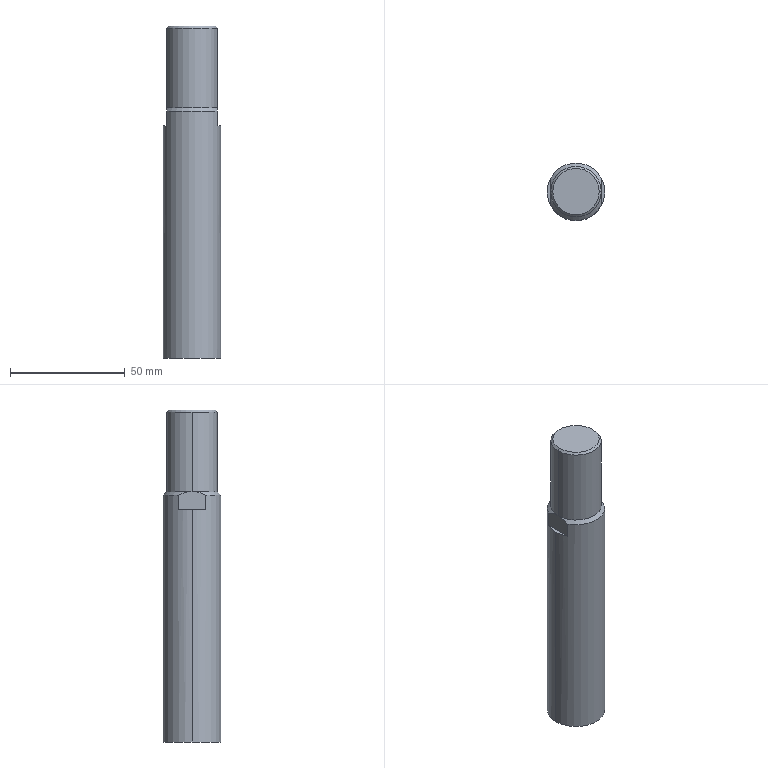Part | STEP file | A_CDQ2A80-100DM-F9NV (Rod) | 1 solid | 14 faces | box 25 x 25 x 144.5 mm | volume 66720 mm3 | cone 4 | cylinder 4 | plane 4 | spline 2 | commonest cylinder face diameters 22 x2 25 x2
STEP:
#1=CARTESIAN_POINT('',(0.,0.,0.));
#2=DIRECTION('',(0.,0.,1.));
#3=DIRECTION('',(1.,0.,0.));
#4=AXIS2_PLACEMENT_3D('',#1,#2,#3);
#5=CARTESIAN_POINT('',(-10.105,0.,43.5));
#6=VERTEX_POINT('',#5);
#7=CARTESIAN_POINT('',(10.105,0.,43.5));
#8=VERTEX_POINT('',#7);
#9=CARTESIAN_POINT('',(0.,0.,43.5));
#10=DIRECTION('',(0.,0.,-1.));
#11=DIRECTION('',(-1.,0.,0.));
#12=AXIS2_PLACEMENT_3D('',#9,#10,#11);
#13=CIRCLE('',#12,10.105);
#14=CARTESIAN_POINT('',(0.,0.,43.5));
#15=DIRECTION('',(0.,0.,-1.));
#16=DIRECTION('',(-1.,0.,0.));
#17=AXIS2_PLACEMENT_3D('',#14,#15,#16);
#18=CONICAL_SURFACE('',#17,10.105,0.7854);
#19=CARTESIAN_POINT('',(0.,0.));
#20=DIRECTION('',(1.,0.));
#21=VECTOR('',#20,1.);
#22=LINE('',#19,#21);
#23=(GEOMETRIC_REPRESENTATION_CONTEXT(2)PARAMETRIC_REPRESENTATION_CONTEXT()REPRESENTATION_CONTEXT('',''));
#24=DEFINITIONAL_REPRESENTATION('',(#22),#23);
#25=PCURVE('',#18,#24);
#26=CARTESIAN_POINT('',(10.226,-10.105,43.5));
#27=DIRECTION('',(0.,0.,1.));
#28=DIRECTION('',(0.,1.,0.));
#29=AXIS2_PLACEMENT_3D('',#26,#27,#28);
#30=PLANE('',#29);
#31=CARTESIAN_POINT('',(10.105,20.331));
#32=CARTESIAN_POINT('',(27.607,20.331));
#33=CARTESIAN_POINT('',(18.856,5.174));
#34=CARTESIAN_POINT('',(10.105,-9.984));
#35=CARTESIAN_POINT('',(1.354,5.174));
#36=CARTESIAN_POINT('',(-7.397,20.331));
#37=CARTESIAN_POINT('',(10.105,20.331));
#38=(BOUNDED_CURVE()B_SPLINE_CURVE(2,(#31,#32,#33,#34,#35,#36,#37),.UNSPECIFIED.,.T.,.F.)B_SPLINE_CURVE_WITH_KNOTS((1,2,2,2,2,1),(-2.094,0.,2.094,4.189,6.283,8.378),.UNSPECIFIED.)CURVE()GEOMETRIC_REPRESENTATION_ITEM()RATIONAL_B_SPLINE_CURVE((1.,0.5,1.,0.5,1.,0.5,1.))REPRESENTATION_ITEM(''));
#39=(GEOMETRIC_REPRESENTATION_CONTEXT(2)PARAMETRIC_REPRESENTATION_CONTEXT()REPRESENTATION_CONTEXT('',''));
#40=DEFINITIONAL_REPRESENTATION('',(#38),#39);
#41=PCURVE('',#30,#40);
#42=SURFACE_CURVE('',#13,(#25,#41),.PCURVE_S1.);
#43=EDGE_CURVE('',#6,#8,#42,.T.);
#44=ORIENTED_EDGE('',*,*,#43,.T.);
#45=CARTESIAN_POINT('',(11.,0.,42.605));
#46=VERTEX_POINT('',#45);
#47=CARTESIAN_POINT('',(10.105,0.,43.5));
#48=DIRECTION('',(0.7071,0.,-0.7071));
#49=VECTOR('',#48,1.);
#50=LINE('',#47,#49);
#51=CARTESIAN_POINT('',(3.142,0.));
#52=DIRECTION('',(0.,1.));
#53=VECTOR('',#52,1.);
#54=LINE('',#51,#53);
#55=(GEOMETRIC_REPRESENTATION_CONTEXT(2)PARAMETRIC_REPRESENTATION_CONTEXT()REPRESENTATION_CONTEXT('',''));
#56=DEFINITIONAL_REPRESENTATION('',(#54),#55);
#57=PCURVE('',#18,#56);
#58=CARTESIAN_POINT('',(0.,0.,43.5));
#59=DIRECTION('',(0.,0.,-1.));
#60=DIRECTION('',(-1.,0.,0.));
#61=AXIS2_PLACEMENT_3D('',#58,#59,#60);
#62=CONICAL_SURFACE('',#61,10.105,0.7854);
#63=CARTESIAN_POINT('',(3.142,0.));
#64=DIRECTION('',(0.,1.));
#65=VECTOR('',#64,1.);
#66=LINE('',#63,#65);
#67=(GEOMETRIC_REPRESENTATION_CONTEXT(2)PARAMETRIC_REPRESENTATION_CONTEXT()REPRESENTATION_CONTEXT('',''));
#68=DEFINITIONAL_REPRESENTATION('',(#66),#67);
#69=PCURVE('',#62,#68);
#70=SURFACE_CURVE('',#50,(#57,#69),.PCURVE_S1.);
#71=EDGE_CURVE('',#8,#46,#70,.T.);
#72=ORIENTED_EDGE('',*,*,#71,.T.);
#73=CARTESIAN_POINT('',(-11.,0.,42.605));
#74=VERTEX_POINT('',#73);
#75=CARTESIAN_POINT('',(0.,0.,42.605));
#76=DIRECTION('',(0.,0.,1.));
#77=DIRECTION('',(0.,1.,0.));
#78=AXIS2_PLACEMENT_3D('',#75,#76,#77);
#79=CIRCLE('',#78,11.);
#80=CARTESIAN_POINT('',(7.854,0.895));
#81=DIRECTION('',(-1.,0.));
#82=VECTOR('',#81,1.);
#83=LINE('',#80,#82);
#84=(GEOMETRIC_REPRESENTATION_CONTEXT(2)PARAMETRIC_REPRESENTATION_CONTEXT()REPRESENTATION_CONTEXT('',''));
#85=DEFINITIONAL_REPRESENTATION('',(#83),#84);
#86=PCURVE('',#18,#85);
#87=CARTESIAN_POINT('',(0.,0.,42.605));
#88=DIRECTION('',(0.,0.,1.));
#89=DIRECTION('',(1.,0.,0.));
#90=AXIS2_PLACEMENT_3D('',#87,#88,#89);
#91=CYLINDRICAL_SURFACE('',#90,11.);
#92=CARTESIAN_POINT('',(-4.712,0.));
#93=DIRECTION('',(1.,0.));
#94=VECTOR('',#93,1.);
#95=LINE('',#92,#94);
#96=(GEOMETRIC_REPRESENTATION_CONTEXT(2)PARAMETRIC_REPRESENTATION_CONTEXT()REPRESENTATION_CONTEXT('',''));
#97=DEFINITIONAL_REPRESENTATION('',(#95),#96);
#98=PCURVE('',#91,#97);
#99=SURFACE_CURVE('',#79,(#86,#98),.PCURVE_S1.);
#100=EDGE_CURVE('',#46,#74,#99,.T.);
#101=ORIENTED_EDGE('',*,*,#100,.T.);
#102=CARTESIAN_POINT('',(-10.105,0.,43.5));
#103=DIRECTION('',(-0.7071,0.,-0.7071));
#104=VECTOR('',#103,1.);
#105=LINE('',#102,#104);
#106=CARTESIAN_POINT('',(0.,0.));
#107=DIRECTION('',(0.,1.));
#108=VECTOR('',#107,1.);
#109=LINE('',#106,#108);
#110=(GEOMETRIC_REPRESENTATION_CONTEXT(2)PARAMETRIC_REPRESENTATION_CONTEXT()REPRESENTATION_CONTEXT('',''));
#111=DEFINITIONAL_REPRESENTATION('',(#109),#110);
#112=PCURVE('',#18,#111);
#113=CARTESIAN_POINT('',(6.283,0.));
#114=DIRECTION('',(0.,1.));
#115=VECTOR('',#114,1.);
#116=LINE('',#113,#115);
#117=(GEOMETRIC_REPRESENTATION_CONTEXT(2)PARAMETRIC_REPRESENTATION_CONTEXT()REPRESENTATION_CONTEXT('',''));
#118=DEFINITIONAL_REPRESENTATION('',(#116),#117);
#119=PCURVE('',#62,#118);
#120=SURFACE_CURVE('',#105,(#112,#119),.PCURVE_S1.);
#121=EDGE_CURVE('',#6,#74,#120,.T.);
#122=ORIENTED_EDGE('',*,*,#121,.F.);
#123=EDGE_LOOP('',(#44,#72,#101,#122));
#124=FACE_BOUND('',#123,.T.);
#125=ADVANCED_FACE('',(#124),#18,.T.);
#126=CARTESIAN_POINT('',(11.,0.,8.));
#127=VERTEX_POINT('',#126);
#128=CARTESIAN_POINT('',(-11.,0.,8.));
#129=VERTEX_POINT('',#128);
#130=CARTESIAN_POINT('',(0.,0.,8.));
#131=DIRECTION('',(0.,0.,1.));
#132=DIRECTION('',(0.,1.,0.));
#133=AXIS2_PLACEMENT_3D('',#130,#131,#132);
#134=CIRCLE('',#133,11.);
#135=CARTESIAN_POINT('',(-4.712,-34.605));
#136=DIRECTION('',(1.,0.));
#137=VECTOR('',#136,1.);
#138=LINE('',#135,#137);
#139=(GEOMETRIC_REPRESENTATION_CONTEXT(2)PARAMETRIC_REPRESENTATION_CONTEXT()REPRESENTATION_CONTEXT('',''));
#140=DEFINITIONAL_REPRESENTATION('',(#138),#139);
#141=PCURVE('',#91,#140);
#142=CARTESIAN_POINT('',(0.,0.,8.));
#143=DIRECTION('',(0.,0.,-1.));
#144=DIRECTION('',(-1.,0.,0.));
#145=AXIS2_PLACEMENT_3D('',#142,#143,#144);
#146=CONICAL_SURFACE('',#145,11.,0.7854);
#147=CARTESIAN_POINT('',(7.854,0.));
#148=DIRECTION('',(-1.,0.));
#149=VECTOR('',#148,1.);
#150=LINE('',#147,#149);
#151=(GEOMETRIC_REPRESENTATION_CONTEXT(2)PARAMETRIC_REPRESENTATION_CONTEXT()REPRESENTATION_CONTEXT('',''));
#152=DEFINITIONAL_REPRESENTATION('',(#150),#151);
#153=PCURVE('',#146,#152);
#154=SURFACE_CURVE('',#134,(#141,#153),.PCURVE_S1.);
#155=EDGE_CURVE('',#127,#129,#154,.T.);
#156=ORIENTED_EDGE('',*,*,#155,.T.);
#157=CARTESIAN_POINT('',(-11.,0.,42.605));
#158=DIRECTION('',(0.,0.,1.));
#159=VECTOR('',#158,1.);
#160=LINE('',#157,#159);
#161=CARTESIAN_POINT('',(3.142,0.));
#162=DIRECTION('',(0.,1.));
#163=VECTOR('',#162,1.);
#164=LINE('',#161,#163);
#165=(GEOMETRIC_REPRESENTATION_CONTEXT(2)PARAMETRIC_REPRESENTATION_CONTEXT()REPRESENTATION_CONTEXT('',''));
#166=DEFINITIONAL_REPRESENTATION('',(#164),#165);
#167=PCURVE('',#91,#166);
#168=CARTESIAN_POINT('',(0.,0.,42.605));
#169=DIRECTION('',(0.,0.,1.));
#170=DIRECTION('',(1.,0.,0.));
#171=AXIS2_PLACEMENT_3D('',#168,#169,#170);
#172=CYLINDRICAL_SURFACE('',#171,11.);
#173=CARTESIAN_POINT('',(3.142,0.));
#174=DIRECTION('',(0.,1.));
#175=VECTOR('',#174,1.);
#176=LINE('',#173,#175);
#177=(GEOMETRIC_REPRESENTATION_CONTEXT(2)PARAMETRIC_REPRESENTATION_CONTEXT()REPRESENTATION_CONTEXT('',''));
#178=DEFINITIONAL_REPRESENTATION('',(#176),#177);
#179=PCURVE('',#172,#178);
#180=SURFACE_CURVE('',#160,(#167,#179),.PCURVE_S1.);
#181=EDGE_CURVE('',#129,#74,#180,.T.);
#182=ORIENTED_EDGE('',*,*,#181,.T.);
#183=ORIENTED_EDGE('',*,*,#100,.F.);
#184=CARTESIAN_POINT('',(11.,0.,42.605));
#185=DIRECTION('',(0.,0.,1.));
#186=VECTOR('',#185,1.);
#187=LINE('',#184,#186);
#188=CARTESIAN_POINT('',(0.,0.));
#189=DIRECTION('',(0.,1.));
#190=VECTOR('',#189,1.);
#191=LINE('',#188,#190);
#192=(GEOMETRIC_REPRESENTATION_CONTEXT(2)PARAMETRIC_REPRESENTATION_CONTEXT()REPRESENTATION_CONTEXT('',''));
#193=DEFINITIONAL_REPRESENTATION('',(#191),#192);
#194=PCURVE('',#91,#193);
#195=CARTESIAN_POINT('',(6.283,0.));
#196=DIRECTION('',(0.,1.));
#197=VECTOR('',#196,1.);
#198=LINE('',#195,#197);
#199=(GEOMETRIC_REPRESENTATION_CONTEXT(2)PARAMETRIC_REPRESENTATION_CONTEXT()REPRESENTATION_CONTEXT('',''));
#200=DEFINITIONAL_REPRESENTATION('',(#198),#199);
#201=PCURVE('',#172,#200);
#202=SURFACE_CURVE('',#187,(#194,#201),.PCURVE_S1.);
#203=EDGE_CURVE('',#127,#46,#202,.T.);
#204=ORIENTED_EDGE('',*,*,#203,.F.);
#205=EDGE_LOOP('',(#156,#182,#183,#204));
#206=FACE_BOUND('',#205,.T.);
#207=ADVANCED_FACE('',(#206),#91,.T.);
#208=CARTESIAN_POINT('',(12.5,0.,-101.));
#209=VERTEX_POINT('',#208);
#210=CARTESIAN_POINT('',(-12.5,0.,-101.));
#211=VERTEX_POINT('',#210);
#212=CARTESIAN_POINT('',(0.,0.,-101.));
#213=DIRECTION('',(0.,0.,1.));
#214=DIRECTION('',(1.,0.,0.));
#215=AXIS2_PLACEMENT_3D('',#212,#213,#214);
#216=CIRCLE('',#215,12.5);
#217=CARTESIAN_POINT('',(0.,0.,6.5));
#218=DIRECTION('',(0.,0.,1.));
#219=DIRECTION('',(1.,0.,0.));
#220=AXIS2_PLACEMENT_3D('',#217,#218,#219);
#221=CYLINDRICAL_SURFACE('',#220,12.5);
#222=CARTESIAN_POINT('',(0.,-107.5));
#223=DIRECTION('',(1.,0.));
#224=VECTOR('',#223,1.);
#225=LINE('',#222,#224);
#226=(GEOMETRIC_REPRESENTATION_CONTEXT(2)PARAMETRIC_REPRESENTATION_CONTEXT()REPRESENTATION_CONTEXT('',''));
#227=DEFINITIONAL_REPRESENTATION('',(#225),#226);
#228=PCURVE('',#221,#227);
#229=CARTESIAN_POINT('',(12.65,12.5,-101.));
#230=DIRECTION('',(0.,0.,-1.));
#231=DIRECTION('',(0.,-1.,0.));
#232=AXIS2_PLACEMENT_3D('',#229,#230,#231);
#233=PLANE('',#232);
#234=CARTESIAN_POINT('',(12.5,0.15));
#235=CARTESIAN_POINT('',(-9.151,0.15));
#236=CARTESIAN_POINT('',(1.675,18.9));
#237=CARTESIAN_POINT('',(12.5,37.65));
#238=CARTESIAN_POINT('',(23.325,18.9));
#239=CARTESIAN_POINT('',(34.151,0.15));
#240=CARTESIAN_POINT('',(12.5,0.15));
#241=(BOUNDED_CURVE()B_SPLINE_CURVE(2,(#234,#235,#236,#237,#238,#239,#240),.UNSPECIFIED.,.T.,.F.)B_SPLINE_CURVE_WITH_KNOTS((1,2,2,2,2,1),(-2.094,0.,2.094,4.189,6.283,8.378),.UNSPECIFIED.)CURVE()GEOMETRIC_REPRESENTATION_ITEM()RATIONAL_B_SPLINE_CURVE((1.,0.5,1.,0.5,1.,0.5,1.))REPRESENTATION_ITEM(''));
#242=(GEOMETRIC_REPRESENTATION_CONTEXT(2)PARAMETRIC_REPRESENTATION_CONTEXT()REPRESENTATION_CONTEXT('',''));
#243=DEFINITIONAL_REPRESENTATION('',(#241),#242);
#244=PCURVE('',#233,#243);
#245=SURFACE_CURVE('',#216,(#228,#244),.PCURVE_S1.);
#246=EDGE_CURVE('',#209,#211,#245,.T.);
#247=ORIENTED_EDGE('',*,*,#246,.T.);
#248=CARTESIAN_POINT('',(-12.5,0.,0.1));
#249=VERTEX_POINT('',#248);
#250=CARTESIAN_POINT('',(-12.5,0.,6.5));
#251=DIRECTION('',(0.,0.,1.));
#252=VECTOR('',#251,1.);
#253=LINE('',#250,#252);
#254=CARTESIAN_POINT('',(3.142,0.));
#255=DIRECTION('',(0.,1.));
#256=VECTOR('',#255,1.);
#257=LINE('',#254,#256);
#258=(GEOMETRIC_REPRESENTATION_CONTEXT(2)PARAMETRIC_REPRESENTATION_CONTEXT()REPRESENTATION_CONTEXT('',''));
#259=DEFINITIONAL_REPRESENTATION('',(#257),#258);
#260=PCURVE('',#221,#259);
#261=CARTESIAN_POINT('',(0.,0.,6.5));
#262=DIRECTION('',(0.,0.,1.));
#263=DIRECTION('',(1.,0.,0.));
#264=AXIS2_PLACEMENT_3D('',#261,#262,#263);
#265=CYLINDRICAL_SURFACE('',#264,12.5);
#266=CARTESIAN_POINT('',(3.142,0.));
#267=DIRECTION('',(0.,1.));
#268=VECTOR('',#267,1.);
#269=LINE('',#266,#268);
#270=(GEOMETRIC_REPRESENTATION_CONTEXT(2)PARAMETRIC_REPRESENTATION_CONTEXT()REPRESENTATION_CONTEXT('',''));
#271=DEFINITIONAL_REPRESENTATION('',(#269),#270);
#272=PCURVE('',#265,#271);
#273=SURFACE_CURVE('',#253,(#260,#272),.PCURVE_S1.);
#274=EDGE_CURVE('',#211,#249,#273,.T.);
#275=ORIENTED_EDGE('',*,*,#274,.T.);
#276=CARTESIAN_POINT('',(-11.,5.937,0.1));
#277=VERTEX_POINT('',#276);
#278=CARTESIAN_POINT('',(0.,0.,0.1));
#279=DIRECTION('',(0.,0.,-1.));
#280=DIRECTION('',(1.,0.,0.));
#281=AXIS2_PLACEMENT_3D('',#278,#279,#280);
#282=CIRCLE('',#281,12.5);
#283=CARTESIAN_POINT('',(6.283,-6.4));
#284=DIRECTION('',(-1.,0.));
#285=VECTOR('',#284,1.);
#286=LINE('',#283,#285);
#287=(GEOMETRIC_REPRESENTATION_CONTEXT(2)PARAMETRIC_REPRESENTATION_CONTEXT()REPRESENTATION_CONTEXT('',''));
#288=DEFINITIONAL_REPRESENTATION('',(#286),#287);
#289=PCURVE('',#221,#288);
#290=CARTESIAN_POINT('',(-12.689,-6.008,0.1));
#291=CARTESIAN_POINT('',(-12.689,6.008,0.1));
#292=CARTESIAN_POINT('',(-12.515,-6.008,0.1));
#293=CARTESIAN_POINT('',(-12.515,6.008,0.1));
#294=CARTESIAN_POINT('',(-12.5,-6.008,0.1));
#295=CARTESIAN_POINT('',(-12.5,6.008,0.1));
#296=CARTESIAN_POINT('',(-11.,-6.008,0.1));
#297=CARTESIAN_POINT('',(-11.,6.008,0.1));
#298=B_SPLINE_SURFACE_WITH_KNOTS('',1,1,((#290,#291),(#292,#293),(#294,#295),(#296,#297)),.UNSPECIFIED.,.F.,.F.,.F.,(2,1,1,2),(2,2),(-0.1261,-0.01,0.,1.),(0.,1.),.UNSPECIFIED.);
#299=CARTESIAN_POINT('',(0.,0.5));
#300=CARTESIAN_POINT('',(-0.000000178,0.5078));
#301=CARTESIAN_POINT('',(0.001406,0.5234));
#302=CARTESIAN_POINT('',(0.007732,0.5468));
#303=CARTESIAN_POINT('',(0.01827,0.5702));
#304=CARTESIAN_POINT('',(0.03302,0.5935));
#305=CARTESIAN_POINT('',(0.05197,0.6168));
#306=CARTESIAN_POINT('',(0.07511,0.64));
#307=CARTESIAN_POINT('',(0.1024,0.6631));
#308=CARTESIAN_POINT('',(0.1339,0.6862));
#309=CARTESIAN_POINT('',(0.1695,0.7092));
#310=CARTESIAN_POINT('',(0.2093,0.7321));
#311=CARTESIAN_POINT('',(0.2532,0.7548));
#312=CARTESIAN_POINT('',(0.3012,0.7774));
#313=CARTESIAN_POINT('',(0.3532,0.7999));
#314=CARTESIAN_POINT('',(0.4093,0.8223));
#315=CARTESIAN_POINT('',(0.4693,0.8444));
#316=CARTESIAN_POINT('',(0.5334,0.8664));
#317=CARTESIAN_POINT('',(0.6014,0.8882));
#318=CARTESIAN_POINT('',(0.6733,0.9098));
#319=CARTESIAN_POINT('',(0.7491,0.9312));
#320=CARTESIAN_POINT('',(0.8288,0.9524));
#321=CARTESIAN_POINT('',(0.9122,0.9734));
#322=CARTESIAN_POINT('',(0.9703,0.9872));
#323=CARTESIAN_POINT('',(1.,0.9941));
#324=B_SPLINE_CURVE_WITH_KNOTS('',3,(#299,#300,#301,#302,#303,#304,#305,#306,#307,#308,#309,#310,#311,#312,#313,#314,#315,#316,#317,#318,#319,#320,#321,#322,#323),.UNSPECIFIED.,.F.,.F.,(4,1,1,1,1,1,1,1,1,1,1,1,1,1,1,1,1,1,1,1,1,1,4),(3.142,3.164,3.187,3.209,3.232,3.254,3.277,3.299,3.322,3.344,3.367,3.389,3.412,3.434,3.457,3.479,3.502,3.524,3.547,3.569,3.592,3.614,3.637),.QUASI_UNIFORM_KNOTS.);
#325=(GEOMETRIC_REPRESENTATION_CONTEXT(2)PARAMETRIC_REPRESENTATION_CONTEXT()REPRESENTATION_CONTEXT('',''));
#326=DEFINITIONAL_REPRESENTATION('',(#324),#325);
#327=PCURVE('',#298,#326);
#328=SURFACE_CURVE('',#282,(#289,#327),.PCURVE_S1.);
#329=EDGE_CURVE('',#249,#277,#328,.T.);
#330=ORIENTED_EDGE('',*,*,#329,.T.);
#331=CARTESIAN_POINT('',(-11.,5.937,6.5));
#332=VERTEX_POINT('',#331);
#333=CARTESIAN_POINT('',(-11.,5.937,-47.25));
#334=DIRECTION('',(0.,0.,1.));
#335=VECTOR('',#334,1.);
#336=LINE('',#333,#335);
#337=CARTESIAN_POINT('',(2.647,-53.75));
#338=DIRECTION('',(0.,1.));
#339=VECTOR('',#338,1.);
#340=LINE('',#337,#339);
#341=(GEOMETRIC_REPRESENTATION_CONTEXT(2)PARAMETRIC_REPRESENTATION_CONTEXT()REPRESENTATION_CONTEXT('',''));
#342=DEFINITIONAL_REPRESENTATION('',(#340),#341);
#343=PCURVE('',#221,#342);
#344=CARTESIAN_POINT('',(-11.,-5.937,8.047));
#345=DIRECTION('',(-1.,0.,0.));
#346=DIRECTION('',(0.,1.,0.));
#347=AXIS2_PLACEMENT_3D('',#344,#345,#346);
#348=PLANE('',#347);
#349=CARTESIAN_POINT('',(11.874,55.297));
#350=DIRECTION('',(0.,-1.));
#351=VECTOR('',#350,1.);
#352=LINE('',#349,#351);
#353=(GEOMETRIC_REPRESENTATION_CONTEXT(2)PARAMETRIC_REPRESENTATION_CONTEXT()REPRESENTATION_CONTEXT('',''));
#354=DEFINITIONAL_REPRESENTATION('',(#352),#353);
#355=PCURVE('',#348,#354);
#356=SURFACE_CURVE('',#336,(#343,#355),.PCURVE_S1.);
#357=EDGE_CURVE('',#277,#332,#356,.T.);
#358=ORIENTED_EDGE('',*,*,#357,.T.);
#359=CARTESIAN_POINT('',(11.,5.937,6.5));
#360=VERTEX_POINT('',#359);
#361=CARTESIAN_POINT('',(0.,0.,6.5));
#362=DIRECTION('',(0.,0.,1.));
#363=DIRECTION('',(0.,1.,0.));
#364=AXIS2_PLACEMENT_3D('',#361,#362,#363);
#365=CIRCLE('',#364,12.5);
#366=CARTESIAN_POINT('',(-4.712,0.));
#367=DIRECTION('',(1.,0.));
#368=VECTOR('',#367,1.);
#369=LINE('',#366,#368);
#370=(GEOMETRIC_REPRESENTATION_CONTEXT(2)PARAMETRIC_REPRESENTATION_CONTEXT()REPRESENTATION_CONTEXT('',''));
#371=DEFINITIONAL_REPRESENTATION('',(#369),#370);
#372=PCURVE('',#221,#371);
#373=CARTESIAN_POINT('',(7.854,1.5));
#374=DIRECTION('',(-1.,0.));
#375=VECTOR('',#374,1.);
#376=LINE('',#373,#375);
#377=(GEOMETRIC_REPRESENTATION_CONTEXT(2)PARAMETRIC_REPRESENTATION_CONTEXT()REPRESENTATION_CONTEXT('',''));
#378=DEFINITIONAL_REPRESENTATION('',(#376),#377);
#379=PCURVE('',#146,#378);
#380=SURFACE_CURVE('',#365,(#372,#379),.PCURVE_S1.);
#381=EDGE_CURVE('',#360,#332,#380,.T.);
#382=ORIENTED_EDGE('',*,*,#381,.F.);
#383=CARTESIAN_POINT('',(11.,5.937,0.1));
#384=VERTEX_POINT('',#383);
#385=CARTESIAN_POINT('',(11.,5.937,-47.25));
#386=DIRECTION('',(0.,0.,-1.));
#387=VECTOR('',#386,1.);
#388=LINE('',#385,#387);
#389=CARTESIAN_POINT('',(0.4949,-53.75));
#390=DIRECTION('',(0.,-1.));
#391=VECTOR('',#390,1.);
#392=LINE('',#389,#391);
#393=(GEOMETRIC_REPRESENTATION_CONTEXT(2)PARAMETRIC_REPRESENTATION_CONTEXT()REPRESENTATION_CONTEXT('',''));
#394=DEFINITIONAL_REPRESENTATION('',(#392),#393);
#395=PCURVE('',#221,#394);
#396=CARTESIAN_POINT('',(11.,5.937,8.047));
#397=DIRECTION('',(1.,0.,0.));
#398=DIRECTION('',(0.,-1.,0.));
#399=AXIS2_PLACEMENT_3D('',#396,#397,#398);
#400=PLANE('',#399);
#401=CARTESIAN_POINT('',(0.,55.297));
#402=DIRECTION('',(0.,1.));
#403=VECTOR('',#402,1.);
#404=LINE('',#401,#403);
#405=(GEOMETRIC_REPRESENTATION_CONTEXT(2)PARAMETRIC_REPRESENTATION_CONTEXT()REPRESENTATION_CONTEXT('',''));
#406=DEFINITIONAL_REPRESENTATION('',(#404),#405);
#407=PCURVE('',#400,#406);
#408=SURFACE_CURVE('',#388,(#395,#407),.PCURVE_S1.);
#409=EDGE_CURVE('',#360,#384,#408,.T.);
#410=ORIENTED_EDGE('',*,*,#409,.T.);
#411=CARTESIAN_POINT('',(12.5,0.,0.1));
#412=VERTEX_POINT('',#411);
#413=CARTESIAN_POINT('',(0.,0.,0.1));
#414=DIRECTION('',(0.,0.,-1.));
#415=DIRECTION('',(1.,0.,0.));
#416=AXIS2_PLACEMENT_3D('',#413,#414,#415);
#417=CIRCLE('',#416,12.5);
#418=CARTESIAN_POINT('',(6.283,-6.4));
#419=DIRECTION('',(-1.,0.));
#420=VECTOR('',#419,1.);
#421=LINE('',#418,#420);
#422=(GEOMETRIC_REPRESENTATION_CONTEXT(2)PARAMETRIC_REPRESENTATION_CONTEXT()REPRESENTATION_CONTEXT('',''));
#423=DEFINITIONAL_REPRESENTATION('',(#421),#422);
#424=PCURVE('',#221,#423);
#425=CARTESIAN_POINT('',(11.,-6.008,0.1));
#426=CARTESIAN_POINT('',(11.,6.008,0.1));
#427=CARTESIAN_POINT('',(12.5,-6.008,0.1));
#428=CARTESIAN_POINT('',(12.5,6.008,0.1));
#429=CARTESIAN_POINT('',(12.515,-6.008,0.1));
#430=CARTESIAN_POINT('',(12.515,6.008,0.1));
#431=CARTESIAN_POINT('',(12.689,-6.008,0.1));
#432=CARTESIAN_POINT('',(12.689,6.008,0.1));
#433=B_SPLINE_SURFACE_WITH_KNOTS('',1,1,((#425,#426),(#427,#428),(#429,#430),(#431,#432)),.UNSPECIFIED.,.F.,.F.,.F.,(2,1,1,2),(2,2),(0.,1.,1.01,1.126),(0.,1.),.UNSPECIFIED.);
#434=CARTESIAN_POINT('',(0.,0.9941));
#435=CARTESIAN_POINT('',(0.02968,0.9872));
#436=CARTESIAN_POINT('',(0.08781,0.9734));
#437=CARTESIAN_POINT('',(0.1712,0.9524));
#438=CARTESIAN_POINT('',(0.2509,0.9312));
#439=CARTESIAN_POINT('',(0.3267,0.9098));
#440=CARTESIAN_POINT('',(0.3986,0.8882));
#441=CARTESIAN_POINT('',(0.4666,0.8664));
#442=CARTESIAN_POINT('',(0.5307,0.8444));
#443=CARTESIAN_POINT('',(0.5907,0.8223));
#444=CARTESIAN_POINT('',(0.6468,0.7999));
#445=CARTESIAN_POINT('',(0.6988,0.7774));
#446=CARTESIAN_POINT('',(0.7468,0.7548));
#447=CARTESIAN_POINT('',(0.7907,0.7321));
#448=CARTESIAN_POINT('',(0.8305,0.7092));
#449=CARTESIAN_POINT('',(0.8661,0.6862));
#450=CARTESIAN_POINT('',(0.8976,0.6631));
#451=CARTESIAN_POINT('',(0.9249,0.64));
#452=CARTESIAN_POINT('',(0.948,0.6168));
#453=CARTESIAN_POINT('',(0.967,0.5935));
#454=CARTESIAN_POINT('',(0.9817,0.5702));
#455=CARTESIAN_POINT('',(0.9923,0.5468));
#456=CARTESIAN_POINT('',(0.9986,0.5234));
#457=CARTESIAN_POINT('',(1.,0.5078));
#458=CARTESIAN_POINT('',(1.,0.5));
#459=B_SPLINE_CURVE_WITH_KNOTS('',3,(#434,#435,#436,#437,#438,#439,#440,#441,#442,#443,#444,#445,#446,#447,#448,#449,#450,#451,#452,#453,#454,#455,#456,#457,#458),.UNSPECIFIED.,.F.,.F.,(4,1,1,1,1,1,1,1,1,1,1,1,1,1,1,1,1,1,1,1,1,1,4),(5.788,5.811,5.833,5.856,5.878,5.901,5.923,5.946,5.968,5.991,6.013,6.036,6.058,6.081,6.103,6.126,6.148,6.171,6.193,6.216,6.238,6.261,6.283),.QUASI_UNIFORM_KNOTS.);
#460=(GEOMETRIC_REPRESENTATION_CONTEXT(2)PARAMETRIC_REPRESENTATION_CONTEXT()REPRESENTATION_CONTEXT('',''));
#461=DEFINITIONAL_REPRESENTATION('',(#459),#460);
#462=PCURVE('',#433,#461);
#463=SURFACE_CURVE('',#417,(#424,#462),.PCURVE_S1.);
#464=EDGE_CURVE('',#384,#412,#463,.T.);
#465=ORIENTED_EDGE('',*,*,#464,.T.);
#466=CARTESIAN_POINT('',(12.5,0.,6.5));
#467=DIRECTION('',(0.,0.,1.));
#468=VECTOR('',#467,1.);
#469=LINE('',#466,#468);
#470=CARTESIAN_POINT('',(0.,0.));
#471=DIRECTION('',(0.,1.));
#472=VECTOR('',#471,1.);
#473=LINE('',#470,#472);
#474=(GEOMETRIC_REPRESENTATION_CONTEXT(2)PARAMETRIC_REPRESENTATION_CONTEXT()REPRESENTATION_CONTEXT('',''));
#475=DEFINITIONAL_REPRESENTATION('',(#473),#474);
#476=PCURVE('',#221,#475);
#477=CARTESIAN_POINT('',(6.283,0.));
#478=DIRECTION('',(0.,1.));
#479=VECTOR('',#478,1.);
#480=LINE('',#477,#479);
#481=(GEOMETRIC_REPRESENTATION_CONTEXT(2)PARAMETRIC_REPRESENTATION_CONTEXT()REPRESENTATION_CONTEXT('',''));
#482=DEFINITIONAL_REPRESENTATION('',(#480),#481);
#483=PCURVE('',#265,#482);
#484=SURFACE_CURVE('',#469,(#476,#483),.PCURVE_S1.);
#485=EDGE_CURVE('',#209,#412,#484,.T.);
#486=ORIENTED_EDGE('',*,*,#485,.F.);
#487=EDGE_LOOP('',(#247,#275,#330,#358,#382,#410,#465,#486));
#488=FACE_BOUND('',#487,.T.);
#489=ADVANCED_FACE('',(#488),#221,.T.);
#490=ORIENTED_EDGE('',*,*,#71,.F.);
#491=CARTESIAN_POINT('',(0.,0.,43.5));
#492=DIRECTION('',(0.,0.,-1.));
#493=DIRECTION('',(-1.,0.,0.));
#494=AXIS2_PLACEMENT_3D('',#491,#492,#493);
#495=CIRCLE('',#494,10.105);
#496=CARTESIAN_POINT('',(0.,0.));
#497=DIRECTION('',(1.,0.));
#498=VECTOR('',#497,1.);
#499=LINE('',#496,#498);
#500=(GEOMETRIC_REPRESENTATION_CONTEXT(2)PARAMETRIC_REPRESENTATION_CONTEXT()REPRESENTATION_CONTEXT('',''));
#501=DEFINITIONAL_REPRESENTATION('',(#499),#500);
#502=PCURVE('',#62,#501);
#503=CARTESIAN_POINT('',(10.105,20.331));
#504=CARTESIAN_POINT('',(27.607,20.331));
#505=CARTESIAN_POINT('',(18.856,5.174));
#506=CARTESIAN_POINT('',(10.105,-9.984));
#507=CARTESIAN_POINT('',(1.354,5.174));
#508=CARTESIAN_POINT('',(-7.397,20.331));
#509=CARTESIAN_POINT('',(10.105,20.331));
#510=(BOUNDED_CURVE()B_SPLINE_CURVE(2,(#503,#504,#505,#506,#507,#508,#509),.UNSPECIFIED.,.T.,.F.)B_SPLINE_CURVE_WITH_KNOTS((1,2,2,2,2,1),(-2.094,0.,2.094,4.189,6.283,8.378),.UNSPECIFIED.)CURVE()GEOMETRIC_REPRESENTATION_ITEM()RATIONAL_B_SPLINE_CURVE((1.,0.5,1.,0.5,1.,0.5,1.))REPRESENTATION_ITEM(''));
#511=(GEOMETRIC_REPRESENTATION_CONTEXT(2)PARAMETRIC_REPRESENTATION_CONTEXT()REPRESENTATION_CONTEXT('',''));
#512=DEFINITIONAL_REPRESENTATION('',(#510),#511);
#513=PCURVE('',#30,#512);
#514=SURFACE_CURVE('',#495,(#502,#513),.PCURVE_S1.);
#515=EDGE_CURVE('',#8,#6,#514,.T.);
#516=ORIENTED_EDGE('',*,*,#515,.T.);
#517=ORIENTED_EDGE('',*,*,#121,.T.);
#518=CARTESIAN_POINT('',(0.,0.,42.605));
#519=DIRECTION('',(0.,0.,1.));
#520=DIRECTION('',(0.,1.,0.));
#521=AXIS2_PLACEMENT_3D('',#518,#519,#520);
#522=CIRCLE('',#521,11.);
#523=CARTESIAN_POINT('',(7.854,0.895));
#524=DIRECTION('',(-1.,0.));
#525=VECTOR('',#524,1.);
#526=LINE('',#523,#525);
#527=(GEOMETRIC_REPRESENTATION_CONTEXT(2)PARAMETRIC_REPRESENTATION_CONTEXT()REPRESENTATION_CONTEXT('',''));
#528=DEFINITIONAL_REPRESENTATION('',(#526),#527);
#529=PCURVE('',#62,#528);
#530=CARTESIAN_POINT('',(1.571,0.));
#531=DIRECTION('',(1.,0.));
#532=VECTOR('',#531,1.);
#533=LINE('',#530,#532);
#534=(GEOMETRIC_REPRESENTATION_CONTEXT(2)PARAMETRIC_REPRESENTATION_CONTEXT()REPRESENTATION_CONTEXT('',''));
#535=DEFINITIONAL_REPRESENTATION('',(#533),#534);
#536=PCURVE('',#172,#535);
#537=SURFACE_CURVE('',#522,(#529,#536),.PCURVE_S1.);
#538=EDGE_CURVE('',#74,#46,#537,.T.);
#539=ORIENTED_EDGE('',*,*,#538,.T.);
#540=EDGE_LOOP('',(#490,#516,#517,#539));
#541=FACE_BOUND('',#540,.T.);
#542=ADVANCED_FACE('',(#541),#62,.T.);
#543=ORIENTED_EDGE('',*,*,#43,.F.);
#544=ORIENTED_EDGE('',*,*,#515,.F.);
#545=EDGE_LOOP('',(#543,#544));
#546=FACE_BOUND('',#545,.T.);
#547=ADVANCED_FACE('',(#546),#30,.T.);
#548=ORIENTED_EDGE('',*,*,#181,.F.);
#549=CARTESIAN_POINT('',(0.,0.,8.));
#550=DIRECTION('',(0.,0.,1.));
#551=DIRECTION('',(0.,1.,0.));
#552=AXIS2_PLACEMENT_3D('',#549,#550,#551);
#553=CIRCLE('',#552,11.);
#554=CARTESIAN_POINT('',(1.571,-34.605));
#555=DIRECTION('',(1.,0.));
#556=VECTOR('',#555,1.);
#557=LINE('',#554,#556);
#558=(GEOMETRIC_REPRESENTATION_CONTEXT(2)PARAMETRIC_REPRESENTATION_CONTEXT()REPRESENTATION_CONTEXT('',''));
#559=DEFINITIONAL_REPRESENTATION('',(#557),#558);
#560=PCURVE('',#172,#559);
#561=CARTESIAN_POINT('',(0.,0.,8.));
#562=DIRECTION('',(0.,0.,-1.));
#563=DIRECTION('',(-1.,0.,0.));
#564=AXIS2_PLACEMENT_3D('',#561,#562,#563);
#565=CONICAL_SURFACE('',#564,11.,0.7854);
#566=CARTESIAN_POINT('',(7.854,0.));
#567=DIRECTION('',(-1.,0.));
#568=VECTOR('',#567,1.);
#569=LINE('',#566,#568);
#570=(GEOMETRIC_REPRESENTATION_CONTEXT(2)PARAMETRIC_REPRESENTATION_CONTEXT()REPRESENTATION_CONTEXT('',''));
#571=DEFINITIONAL_REPRESENTATION('',(#569),#570);
#572=PCURVE('',#565,#571);
#573=SURFACE_CURVE('',#553,(#560,#572),.PCURVE_S1.);
#574=EDGE_CURVE('',#129,#127,#573,.T.);
#575=ORIENTED_EDGE('',*,*,#574,.T.);
#576=ORIENTED_EDGE('',*,*,#203,.T.);
#577=ORIENTED_EDGE('',*,*,#538,.F.);
#578=EDGE_LOOP('',(#548,#575,#576,#577));
#579=FACE_BOUND('',#578,.T.);
#580=ADVANCED_FACE('',(#579),#172,.T.);
#581=CARTESIAN_POINT('',(-11.,-5.937,6.5));
#582=VERTEX_POINT('',#581);
#583=CARTESIAN_POINT('',(-11.,0.,8.));
#584=CARTESIAN_POINT('',(-11.,-1.038,8.));
#585=CARTESIAN_POINT('',(-11.,-2.05,7.852));
#586=CARTESIAN_POINT('',(-11.,-3.538,7.455));
#587=CARTESIAN_POINT('',(-11.,-4.03,7.293));
#588=CARTESIAN_POINT('',(-11.,-4.996,6.927));
#589=CARTESIAN_POINT('',(-11.,-5.47,6.722));
#590=CARTESIAN_POINT('',(-11.,-5.937,6.5));
#591=B_SPLINE_CURVE_WITH_KNOTS('',3,(#583,#584,#585,#586,#587,#588,#589,#590),.UNSPECIFIED.,.F.,.F.,(4,2,2,4),(0.,0.003068,0.004601,0.006135),.UNSPECIFIED.);
#592=CARTESIAN_POINT('',(6.283,0.));
#593=CARTESIAN_POINT('',(6.275,-0.00000044));
#594=CARTESIAN_POINT('',(6.257,0.002441));
#595=CARTESIAN_POINT('',(6.232,0.0133));
#596=CARTESIAN_POINT('',(6.207,0.03123));
#597=CARTESIAN_POINT('',(6.181,0.05608));
#598=CARTESIAN_POINT('',(6.157,0.08773));
#599=CARTESIAN_POINT('',(6.132,0.126));
#600=CARTESIAN_POINT('',(6.108,0.1708));
#601=CARTESIAN_POINT('',(6.083,0.2219));
#602=CARTESIAN_POINT('',(6.06,0.2793));
#603=CARTESIAN_POINT('',(6.036,0.3426));
#604=CARTESIAN_POINT('',(6.013,0.4119));
#605=CARTESIAN_POINT('',(5.991,0.4869));
#606=CARTESIAN_POINT('',(5.968,0.5674));
#607=CARTESIAN_POINT('',(5.946,0.6533));
#608=CARTESIAN_POINT('',(5.925,0.7441));
#609=CARTESIAN_POINT('',(5.904,0.8397));
#610=CARTESIAN_POINT('',(5.884,0.9397));
#611=CARTESIAN_POINT('',(5.864,1.044));
#612=CARTESIAN_POINT('',(5.844,1.152));
#613=CARTESIAN_POINT('',(5.825,1.264));
#614=CARTESIAN_POINT('',(5.806,1.38));
#615=CARTESIAN_POINT('',(5.794,1.46));
#616=CARTESIAN_POINT('',(5.788,1.5));
#617=B_SPLINE_CURVE_WITH_KNOTS('',3,(#592,#593,#594,#595,#596,#597,#598,#599,#600,#601,#602,#603,#604,#605,#606,#607,#608,#609,#610,#611,#612,#613,#614,#615,#616),.UNSPECIFIED.,.F.,.F.,(4,1,1,1,1,1,1,1,1,1,1,1,1,1,1,1,1,1,1,1,1,1,4),(0.,0.0002789,0.0005577,0.0008366,0.001115,0.001394,0.001673,0.001952,0.002231,0.00251,0.002789,0.003068,0.003346,0.003625,0.003904,0.004183,0.004462,0.004741,0.00502,0.005299,0.005577,0.005856,0.006135),.QUASI_UNIFORM_KNOTS.);
#618=(GEOMETRIC_REPRESENTATION_CONTEXT(2)PARAMETRIC_REPRESENTATION_CONTEXT()REPRESENTATION_CONTEXT('',''));
#619=DEFINITIONAL_REPRESENTATION('',(#617),#618);
#620=PCURVE('',#565,#619);
#621=CARTESIAN_POINT('',(5.937,0.0474));
#622=CARTESIAN_POINT('',(4.899,0.0474));
#623=CARTESIAN_POINT('',(3.887,0.1959));
#624=CARTESIAN_POINT('',(2.399,0.5924));
#625=CARTESIAN_POINT('',(1.907,0.754));
#626=CARTESIAN_POINT('',(0.9411,1.121));
#627=CARTESIAN_POINT('',(0.4671,1.326));
#628=CARTESIAN_POINT('',(0.,1.547));
#629=B_SPLINE_CURVE_WITH_KNOTS('',3,(#621,#622,#623,#624,#625,#626,#627,#628),.UNSPECIFIED.,.F.,.F.,(4,2,2,4),(0.,0.003068,0.004601,0.006135),.UNSPECIFIED.);
#630=(GEOMETRIC_REPRESENTATION_CONTEXT(2)PARAMETRIC_REPRESENTATION_CONTEXT()REPRESENTATION_CONTEXT('',''));
#631=DEFINITIONAL_REPRESENTATION('',(#629),#630);
#632=PCURVE('',#348,#631);
#633=SURFACE_CURVE('',#591,(#620,#632),.PCURVE_S1.);
#634=EDGE_CURVE('',#129,#582,#633,.T.);
#635=ORIENTED_EDGE('',*,*,#634,.T.);
#636=CARTESIAN_POINT('',(11.,-5.937,6.5));
#637=VERTEX_POINT('',#636);
#638=CARTESIAN_POINT('',(0.,0.,6.5));
#639=DIRECTION('',(0.,0.,1.));
#640=DIRECTION('',(0.,1.,0.));
#641=AXIS2_PLACEMENT_3D('',#638,#639,#640);
#642=CIRCLE('',#641,12.5);
#643=CARTESIAN_POINT('',(7.854,1.5));
#644=DIRECTION('',(-1.,0.));
#645=VECTOR('',#644,1.);
#646=LINE('',#643,#645);
#647=(GEOMETRIC_REPRESENTATION_CONTEXT(2)PARAMETRIC_REPRESENTATION_CONTEXT()REPRESENTATION_CONTEXT('',''));
#648=DEFINITIONAL_REPRESENTATION('',(#646),#647);
#649=PCURVE('',#565,#648);
#650=CARTESIAN_POINT('',(1.571,0.));
#651=DIRECTION('',(1.,0.));
#652=VECTOR('',#651,1.);
#653=LINE('',#650,#652);
#654=(GEOMETRIC_REPRESENTATION_CONTEXT(2)PARAMETRIC_REPRESENTATION_CONTEXT()REPRESENTATION_CONTEXT('',''));
#655=DEFINITIONAL_REPRESENTATION('',(#653),#654);
#656=PCURVE('',#265,#655);
#657=SURFACE_CURVE('',#642,(#649,#656),.PCURVE_S1.);
#658=EDGE_CURVE('',#582,#637,#657,.T.);
#659=ORIENTED_EDGE('',*,*,#658,.T.);
#660=CARTESIAN_POINT('',(11.,-5.937,6.5));
#661=CARTESIAN_POINT('',(11.,-5.002,6.944));
#662=CARTESIAN_POINT('',(11.,-4.046,7.318));
#663=CARTESIAN_POINT('',(11.,-2.566,7.715));
#664=CARTESIAN_POINT('',(11.,-2.065,7.819));
#665=CARTESIAN_POINT('',(11.,-1.045,7.962));
#666=CARTESIAN_POINT('',(11.,-0.5222,8.));
#667=CARTESIAN_POINT('',(11.,0.,8.));
#668=B_SPLINE_CURVE_WITH_KNOTS('',3,(#660,#661,#662,#663,#664,#665,#666,#667),.UNSPECIFIED.,.F.,.F.,(4,2,2,4),(0.,0.003063,0.004595,0.006127),.UNSPECIFIED.);
#669=CARTESIAN_POINT('',(3.637,1.5));
#670=CARTESIAN_POINT('',(3.631,1.46));
#671=CARTESIAN_POINT('',(3.618,1.38));
#672=CARTESIAN_POINT('',(3.6,1.264));
#673=CARTESIAN_POINT('',(3.581,1.152));
#674=CARTESIAN_POINT('',(3.561,1.045));
#675=CARTESIAN_POINT('',(3.541,0.9408));
#676=CARTESIAN_POINT('',(3.521,0.8415));
#677=CARTESIAN_POINT('',(3.5,0.7468));
#678=CARTESIAN_POINT('',(3.479,0.6567));
#679=CARTESIAN_POINT('',(3.458,0.5716));
#680=CARTESIAN_POINT('',(3.435,0.4915));
#681=CARTESIAN_POINT('',(3.413,0.4167));
#682=CARTESIAN_POINT('',(3.39,0.3473));
#683=CARTESIAN_POINT('',(3.367,0.2836));
#684=CARTESIAN_POINT('',(3.343,0.2258));
#685=CARTESIAN_POINT('',(3.319,0.1741));
#686=CARTESIAN_POINT('',(3.294,0.1286));
#687=CARTESIAN_POINT('',(3.27,0.08961));
#688=CARTESIAN_POINT('',(3.244,0.0573));
#689=CARTESIAN_POINT('',(3.219,0.03189));
#690=CARTESIAN_POINT('',(3.193,0.01357));
#691=CARTESIAN_POINT('',(3.167,0.002485));
#692=CARTESIAN_POINT('',(3.15,-0.000002542));
#693=CARTESIAN_POINT('',(3.142,0.));
#694=B_SPLINE_CURVE_WITH_KNOTS('',3,(#669,#670,#671,#672,#673,#674,#675,#676,#677,#678,#679,#680,#681,#682,#683,#684,#685,#686,#687,#688,#689,#690,#691,#692,#693),.UNSPECIFIED.,.F.,.F.,(4,1,1,1,1,1,1,1,1,1,1,1,1,1,1,1,1,1,1,1,1,1,4),(0.,0.0002785,0.000557,0.0008355,0.001114,0.001392,0.001671,0.001949,0.002228,0.002506,0.002785,0.003063,0.003342,0.00362,0.003899,0.004177,0.004456,0.004734,0.005013,0.005291,0.00557,0.005848,0.006127),.QUASI_UNIFORM_KNOTS.);
#695=(GEOMETRIC_REPRESENTATION_CONTEXT(2)PARAMETRIC_REPRESENTATION_CONTEXT()REPRESENTATION_CONTEXT('',''));
#696=DEFINITIONAL_REPRESENTATION('',(#694),#695);
#697=PCURVE('',#565,#696);
#698=CARTESIAN_POINT('',(11.874,1.547));
#699=CARTESIAN_POINT('',(10.939,1.103));
#700=CARTESIAN_POINT('',(9.983,0.7293));
#701=CARTESIAN_POINT('',(8.504,0.3328));
#702=CARTESIAN_POINT('',(8.003,0.2282));
#703=CARTESIAN_POINT('',(6.982,0.08534));
#704=CARTESIAN_POINT('',(6.459,0.0474));
#705=CARTESIAN_POINT('',(5.937,0.0474));
#706=B_SPLINE_CURVE_WITH_KNOTS('',3,(#698,#699,#700,#701,#702,#703,#704,#705),.UNSPECIFIED.,.F.,.F.,(4,2,2,4),(0.,0.003063,0.004595,0.006127),.UNSPECIFIED.);
#707=(GEOMETRIC_REPRESENTATION_CONTEXT(2)PARAMETRIC_REPRESENTATION_CONTEXT()REPRESENTATION_CONTEXT('',''));
#708=DEFINITIONAL_REPRESENTATION('',(#706),#707);
#709=PCURVE('',#400,#708);
#710=SURFACE_CURVE('',#668,(#697,#709),.PCURVE_S1.);
#711=EDGE_CURVE('',#637,#127,#710,.T.);
#712=ORIENTED_EDGE('',*,*,#711,.T.);
#713=ORIENTED_EDGE('',*,*,#574,.F.);
#714=EDGE_LOOP('',(#635,#659,#712,#713));
#715=FACE_BOUND('',#714,.T.);
#716=ADVANCED_FACE('',(#715),#565,.T.);
#717=CARTESIAN_POINT('',(-11.,5.937,6.5));
#718=CARTESIAN_POINT('',(-11.,5.002,6.944));
#719=CARTESIAN_POINT('',(-11.,4.046,7.318));
#720=CARTESIAN_POINT('',(-11.,2.566,7.715));
#721=CARTESIAN_POINT('',(-11.,2.065,7.819));
#722=CARTESIAN_POINT('',(-11.,1.045,7.962));
#723=CARTESIAN_POINT('',(-11.,0.5222,8.));
#724=CARTESIAN_POINT('',(-11.,0.,8.));
#725=B_SPLINE_CURVE_WITH_KNOTS('',3,(#717,#718,#719,#720,#721,#722,#723,#724),.UNSPECIFIED.,.F.,.F.,(4,2,2,4),(0.,0.003063,0.004595,0.006127),.UNSPECIFIED.);
#726=CARTESIAN_POINT('',(0.4949,1.5));
#727=CARTESIAN_POINT('',(0.4889,1.46));
#728=CARTESIAN_POINT('',(0.4768,1.38));
#729=CARTESIAN_POINT('',(0.4582,1.264));
#730=CARTESIAN_POINT('',(0.4392,1.152));
#731=CARTESIAN_POINT('',(0.4198,1.045));
#732=CARTESIAN_POINT('',(0.3999,0.9408));
#733=CARTESIAN_POINT('',(0.3795,0.8415));
#734=CARTESIAN_POINT('',(0.3588,0.7468));
#735=CARTESIAN_POINT('',(0.3376,0.6567));
#736=CARTESIAN_POINT('',(0.3159,0.5716));
#737=CARTESIAN_POINT('',(0.2939,0.4915));
#738=CARTESIAN_POINT('',(0.2714,0.4167));
#739=CARTESIAN_POINT('',(0.2485,0.3473));
#740=CARTESIAN_POINT('',(0.2251,0.2836));
#741=CARTESIAN_POINT('',(0.2014,0.2258));
#742=CARTESIAN_POINT('',(0.1773,0.1741));
#743=CARTESIAN_POINT('',(0.1529,0.1286));
#744=CARTESIAN_POINT('',(0.128,0.08961));
#745=CARTESIAN_POINT('',(0.1029,0.0573));
#746=CARTESIAN_POINT('',(0.07741,0.03189));
#747=CARTESIAN_POINT('',(0.05172,0.01357));
#748=CARTESIAN_POINT('',(0.0259,0.002485));
#749=CARTESIAN_POINT('',(0.008631,-0.000002542));
#750=CARTESIAN_POINT('',(0.,0.));
#751=B_SPLINE_CURVE_WITH_KNOTS('',3,(#726,#727,#728,#729,#730,#731,#732,#733,#734,#735,#736,#737,#738,#739,#740,#741,#742,#743,#744,#745,#746,#747,#748,#749,#750),.UNSPECIFIED.,.F.,.F.,(4,1,1,1,1,1,1,1,1,1,1,1,1,1,1,1,1,1,1,1,1,1,4),(0.,0.0002785,0.000557,0.0008355,0.001114,0.001392,0.001671,0.001949,0.002228,0.002506,0.002785,0.003063,0.003342,0.00362,0.003899,0.004177,0.004456,0.004734,0.005013,0.005291,0.00557,0.005848,0.006127),.QUASI_UNIFORM_KNOTS.);
#752=(GEOMETRIC_REPRESENTATION_CONTEXT(2)PARAMETRIC_REPRESENTATION_CONTEXT()REPRESENTATION_CONTEXT('',''));
#753=DEFINITIONAL_REPRESENTATION('',(#751),#752);
#754=PCURVE('',#146,#753);
#755=CARTESIAN_POINT('',(11.874,1.547));
#756=CARTESIAN_POINT('',(10.939,1.103));
#757=CARTESIAN_POINT('',(9.983,0.7293));
#758=CARTESIAN_POINT('',(8.504,0.3328));
#759=CARTESIAN_POINT('',(8.003,0.2282));
#760=CARTESIAN_POINT('',(6.982,0.08534));
#761=CARTESIAN_POINT('',(6.459,0.0474));
#762=CARTESIAN_POINT('',(5.937,0.0474));
#763=B_SPLINE_CURVE_WITH_KNOTS('',3,(#755,#756,#757,#758,#759,#760,#761,#762),.UNSPECIFIED.,.F.,.F.,(4,2,2,4),(0.,0.003063,0.004595,0.006127),.UNSPECIFIED.);
#764=(GEOMETRIC_REPRESENTATION_CONTEXT(2)PARAMETRIC_REPRESENTATION_CONTEXT()REPRESENTATION_CONTEXT('',''));
#765=DEFINITIONAL_REPRESENTATION('',(#763),#764);
#766=PCURVE('',#348,#765);
#767=SURFACE_CURVE('',#725,(#754,#766),.PCURVE_S1.);
#768=EDGE_CURVE('',#332,#129,#767,.T.);
#769=ORIENTED_EDGE('',*,*,#768,.T.);
#770=ORIENTED_EDGE('',*,*,#155,.F.);
#771=CARTESIAN_POINT('',(11.,0.,8.));
#772=CARTESIAN_POINT('',(11.,1.038,8.));
#773=CARTESIAN_POINT('',(11.,2.05,7.852));
#774=CARTESIAN_POINT('',(11.,3.538,7.455));
#775=CARTESIAN_POINT('',(11.,4.03,7.293));
#776=CARTESIAN_POINT('',(11.,4.996,6.927));
#777=CARTESIAN_POINT('',(11.,5.47,6.722));
#778=CARTESIAN_POINT('',(11.,5.937,6.5));
#779=B_SPLINE_CURVE_WITH_KNOTS('',3,(#771,#772,#773,#774,#775,#776,#777,#778),.UNSPECIFIED.,.F.,.F.,(4,2,2,4),(0.,0.003068,0.004601,0.006135),.UNSPECIFIED.);
#780=CARTESIAN_POINT('',(3.142,0.));
#781=CARTESIAN_POINT('',(3.133,-0.00000044));
#782=CARTESIAN_POINT('',(3.116,0.002441));
#783=CARTESIAN_POINT('',(3.09,0.0133));
#784=CARTESIAN_POINT('',(3.065,0.03123));
#785=CARTESIAN_POINT('',(3.04,0.05608));
#786=CARTESIAN_POINT('',(3.015,0.08773));
#787=CARTESIAN_POINT('',(2.99,0.126));
#788=CARTESIAN_POINT('',(2.966,0.1708));
#789=CARTESIAN_POINT('',(2.942,0.2219));
#790=CARTESIAN_POINT('',(2.918,0.2793));
#791=CARTESIAN_POINT('',(2.895,0.3426));
#792=CARTESIAN_POINT('',(2.872,0.4119));
#793=CARTESIAN_POINT('',(2.849,0.4869));
#794=CARTESIAN_POINT('',(2.827,0.5674));
#795=CARTESIAN_POINT('',(2.805,0.6533));
#796=CARTESIAN_POINT('',(2.783,0.7441));
#797=CARTESIAN_POINT('',(2.762,0.8397));
#798=CARTESIAN_POINT('',(2.742,0.9397));
#799=CARTESIAN_POINT('',(2.722,1.044));
#800=CARTESIAN_POINT('',(2.702,1.152));
#801=CARTESIAN_POINT('',(2.683,1.264));
#802=CARTESIAN_POINT('',(2.665,1.38));
#803=CARTESIAN_POINT('',(2.653,1.46));
#804=CARTESIAN_POINT('',(2.647,1.5));
#805=B_SPLINE_CURVE_WITH_KNOTS('',3,(#780,#781,#782,#783,#784,#785,#786,#787,#788,#789,#790,#791,#792,#793,#794,#795,#796,#797,#798,#799,#800,#801,#802,#803,#804),.UNSPECIFIED.,.F.,.F.,(4,1,1,1,1,1,1,1,1,1,1,1,1,1,1,1,1,1,1,1,1,1,4),(0.,0.0002789,0.0005577,0.0008366,0.001115,0.001394,0.001673,0.001952,0.002231,0.00251,0.002789,0.003068,0.003346,0.003625,0.003904,0.004183,0.004462,0.004741,0.00502,0.005299,0.005577,0.005856,0.006135),.QUASI_UNIFORM_KNOTS.);
#806=(GEOMETRIC_REPRESENTATION_CONTEXT(2)PARAMETRIC_REPRESENTATION_CONTEXT()REPRESENTATION_CONTEXT('',''));
#807=DEFINITIONAL_REPRESENTATION('',(#805),#806);
#808=PCURVE('',#146,#807);
#809=CARTESIAN_POINT('',(5.937,0.0474));
#810=CARTESIAN_POINT('',(4.899,0.0474));
#811=CARTESIAN_POINT('',(3.887,0.1959));
#812=CARTESIAN_POINT('',(2.399,0.5924));
#813=CARTESIAN_POINT('',(1.907,0.754));
#814=CARTESIAN_POINT('',(0.9411,1.121));
#815=CARTESIAN_POINT('',(0.4671,1.326));
#816=CARTESIAN_POINT('',(0.,1.547));
#817=B_SPLINE_CURVE_WITH_KNOTS('',3,(#809,#810,#811,#812,#813,#814,#815,#816),.UNSPECIFIED.,.F.,.F.,(4,2,2,4),(0.,0.003068,0.004601,0.006135),.UNSPECIFIED.);
#818=(GEOMETRIC_REPRESENTATION_CONTEXT(2)PARAMETRIC_REPRESENTATION_CONTEXT()REPRESENTATION_CONTEXT('',''));
#819=DEFINITIONAL_REPRESENTATION('',(#817),#818);
#820=PCURVE('',#400,#819);
#821=SURFACE_CURVE('',#779,(#808,#820),.PCURVE_S1.);
#822=EDGE_CURVE('',#127,#360,#821,.T.);
#823=ORIENTED_EDGE('',*,*,#822,.T.);
#824=ORIENTED_EDGE('',*,*,#381,.T.);
#825=EDGE_LOOP('',(#769,#770,#823,#824));
#826=FACE_BOUND('',#825,.T.);
#827=ADVANCED_FACE('',(#826),#146,.T.);
#828=ORIENTED_EDGE('',*,*,#274,.F.);
#829=CARTESIAN_POINT('',(0.,0.,-101.));
#830=DIRECTION('',(0.,0.,1.));
#831=DIRECTION('',(1.,0.,0.));
#832=AXIS2_PLACEMENT_3D('',#829,#830,#831);
#833=CIRCLE('',#832,12.5);
#834=CARTESIAN_POINT('',(0.,-107.5));
#835=DIRECTION('',(1.,0.));
#836=VECTOR('',#835,1.);
#837=LINE('',#834,#836);
#838=(GEOMETRIC_REPRESENTATION_CONTEXT(2)PARAMETRIC_REPRESENTATION_CONTEXT()REPRESENTATION_CONTEXT('',''));
#839=DEFINITIONAL_REPRESENTATION('',(#837),#838);
#840=PCURVE('',#265,#839);
#841=CARTESIAN_POINT('',(12.5,0.15));
#842=CARTESIAN_POINT('',(-9.151,0.15));
#843=CARTESIAN_POINT('',(1.675,18.9));
#844=CARTESIAN_POINT('',(12.5,37.65));
#845=CARTESIAN_POINT('',(23.325,18.9));
#846=CARTESIAN_POINT('',(34.151,0.15));
#847=CARTESIAN_POINT('',(12.5,0.15));
#848=(BOUNDED_CURVE()B_SPLINE_CURVE(2,(#841,#842,#843,#844,#845,#846,#847),.UNSPECIFIED.,.T.,.F.)B_SPLINE_CURVE_WITH_KNOTS((1,2,2,2,2,1),(-2.094,0.,2.094,4.189,6.283,8.378),.UNSPECIFIED.)CURVE()GEOMETRIC_REPRESENTATION_ITEM()RATIONAL_B_SPLINE_CURVE((1.,0.5,1.,0.5,1.,0.5,1.))REPRESENTATION_ITEM(''));
#849=(GEOMETRIC_REPRESENTATION_CONTEXT(2)PARAMETRIC_REPRESENTATION_CONTEXT()REPRESENTATION_CONTEXT('',''));
#850=DEFINITIONAL_REPRESENTATION('',(#848),#849);
#851=PCURVE('',#233,#850);
#852=SURFACE_CURVE('',#833,(#840,#851),.PCURVE_S1.);
#853=EDGE_CURVE('',#211,#209,#852,.T.);
#854=ORIENTED_EDGE('',*,*,#853,.T.);
#855=ORIENTED_EDGE('',*,*,#485,.T.);
#856=CARTESIAN_POINT('',(11.,-5.937,0.1));
#857=VERTEX_POINT('',#856);
#858=CARTESIAN_POINT('',(0.,0.,0.1));
#859=DIRECTION('',(0.,0.,-1.));
#860=DIRECTION('',(1.,0.,0.));
#861=AXIS2_PLACEMENT_3D('',#858,#859,#860);
#862=CIRCLE('',#861,12.5);
#863=CARTESIAN_POINT('',(6.283,-6.4));
#864=DIRECTION('',(-1.,0.));
#865=VECTOR('',#864,1.);
#866=LINE('',#863,#865);
#867=(GEOMETRIC_REPRESENTATION_CONTEXT(2)PARAMETRIC_REPRESENTATION_CONTEXT()REPRESENTATION_CONTEXT('',''));
#868=DEFINITIONAL_REPRESENTATION('',(#866),#867);
#869=PCURVE('',#265,#868);
#870=CARTESIAN_POINT('',(1.,0.5));
#871=CARTESIAN_POINT('',(1.,0.4922));
#872=CARTESIAN_POINT('',(0.9986,0.4766));
#873=CARTESIAN_POINT('',(0.9923,0.4532));
#874=CARTESIAN_POINT('',(0.9817,0.4298));
#875=CARTESIAN_POINT('',(0.967,0.4065));
#876=CARTESIAN_POINT('',(0.948,0.3832));
#877=CARTESIAN_POINT('',(0.9249,0.36));
#878=CARTESIAN_POINT('',(0.8976,0.3369));
#879=CARTESIAN_POINT('',(0.8661,0.3138));
#880=CARTESIAN_POINT('',(0.8305,0.2908));
#881=CARTESIAN_POINT('',(0.7907,0.2679));
#882=CARTESIAN_POINT('',(0.7468,0.2452));
#883=CARTESIAN_POINT('',(0.6988,0.2226));
#884=CARTESIAN_POINT('',(0.6468,0.2001));
#885=CARTESIAN_POINT('',(0.5907,0.1777));
#886=CARTESIAN_POINT('',(0.5307,0.1556));
#887=CARTESIAN_POINT('',(0.4666,0.1336));
#888=CARTESIAN_POINT('',(0.3986,0.1118));
#889=CARTESIAN_POINT('',(0.3267,0.09016));
#890=CARTESIAN_POINT('',(0.2509,0.06875));
#891=CARTESIAN_POINT('',(0.1712,0.04756));
#892=CARTESIAN_POINT('',(0.08781,0.02661));
#893=CARTESIAN_POINT('',(0.02968,0.01279));
#894=CARTESIAN_POINT('',(0.,0.005929));
#895=B_SPLINE_CURVE_WITH_KNOTS('',3,(#870,#871,#872,#873,#874,#875,#876,#877,#878,#879,#880,#881,#882,#883,#884,#885,#886,#887,#888,#889,#890,#891,#892,#893,#894),.UNSPECIFIED.,.F.,.F.,(4,1,1,1,1,1,1,1,1,1,1,1,1,1,1,1,1,1,1,1,1,1,4),(0.,0.0225,0.04499,0.06749,0.08999,0.1125,0.135,0.1575,0.18,0.2025,0.225,0.2475,0.27,0.2925,0.315,0.3375,0.36,0.3824,0.4049,0.4274,0.4499,0.4724,0.4949),.QUASI_UNIFORM_KNOTS.);
#896=(GEOMETRIC_REPRESENTATION_CONTEXT(2)PARAMETRIC_REPRESENTATION_CONTEXT()REPRESENTATION_CONTEXT('',''));
#897=DEFINITIONAL_REPRESENTATION('',(#895),#896);
#898=PCURVE('',#433,#897);
#899=SURFACE_CURVE('',#862,(#869,#898),.PCURVE_S1.);
#900=EDGE_CURVE('',#412,#857,#899,.T.);
#901=ORIENTED_EDGE('',*,*,#900,.T.);
#902=CARTESIAN_POINT('',(11.,-5.937,-47.25));
#903=DIRECTION('',(0.,0.,1.));
#904=VECTOR('',#903,1.);
#905=LINE('',#902,#904);
#906=CARTESIAN_POINT('',(5.788,-53.75));
#907=DIRECTION('',(0.,1.));
#908=VECTOR('',#907,1.);
#909=LINE('',#906,#908);
#910=(GEOMETRIC_REPRESENTATION_CONTEXT(2)PARAMETRIC_REPRESENTATION_CONTEXT()REPRESENTATION_CONTEXT('',''));
#911=DEFINITIONAL_REPRESENTATION('',(#909),#910);
#912=PCURVE('',#265,#911);
#913=CARTESIAN_POINT('',(11.874,55.297));
#914=DIRECTION('',(0.,-1.));
#915=VECTOR('',#914,1.);
#916=LINE('',#913,#915);
#917=(GEOMETRIC_REPRESENTATION_CONTEXT(2)PARAMETRIC_REPRESENTATION_CONTEXT()REPRESENTATION_CONTEXT('',''));
#918=DEFINITIONAL_REPRESENTATION('',(#916),#917);
#919=PCURVE('',#400,#918);
#920=SURFACE_CURVE('',#905,(#912,#919),.PCURVE_S1.);
#921=EDGE_CURVE('',#857,#637,#920,.T.);
#922=ORIENTED_EDGE('',*,*,#921,.T.);
#923=ORIENTED_EDGE('',*,*,#658,.F.);
#924=CARTESIAN_POINT('',(-11.,-5.937,0.1));
#925=VERTEX_POINT('',#924);
#926=CARTESIAN_POINT('',(-11.,-5.937,-47.25));
#927=DIRECTION('',(0.,0.,-1.));
#928=VECTOR('',#927,1.);
#929=LINE('',#926,#928);
#930=CARTESIAN_POINT('',(3.637,-53.75));
#931=DIRECTION('',(0.,-1.));
#932=VECTOR('',#931,1.);
#933=LINE('',#930,#932);
#934=(GEOMETRIC_REPRESENTATION_CONTEXT(2)PARAMETRIC_REPRESENTATION_CONTEXT()REPRESENTATION_CONTEXT('',''));
#935=DEFINITIONAL_REPRESENTATION('',(#933),#934);
#936=PCURVE('',#265,#935);
#937=CARTESIAN_POINT('',(0.,55.297));
#938=DIRECTION('',(0.,1.));
#939=VECTOR('',#938,1.);
#940=LINE('',#937,#939);
#941=(GEOMETRIC_REPRESENTATION_CONTEXT(2)PARAMETRIC_REPRESENTATION_CONTEXT()REPRESENTATION_CONTEXT('',''));
#942=DEFINITIONAL_REPRESENTATION('',(#940),#941);
#943=PCURVE('',#348,#942);
#944=SURFACE_CURVE('',#929,(#936,#943),.PCURVE_S1.);
#945=EDGE_CURVE('',#582,#925,#944,.T.);
#946=ORIENTED_EDGE('',*,*,#945,.T.);
#947=CARTESIAN_POINT('',(0.,0.,0.1));
#948=DIRECTION('',(0.,0.,-1.));
#949=DIRECTION('',(1.,0.,0.));
#950=AXIS2_PLACEMENT_3D('',#947,#948,#949);
#951=CIRCLE('',#950,12.5);
#952=CARTESIAN_POINT('',(6.283,-6.4));
#953=DIRECTION('',(-1.,0.));
#954=VECTOR('',#953,1.);
#955=LINE('',#952,#954);
#956=(GEOMETRIC_REPRESENTATION_CONTEXT(2)PARAMETRIC_REPRESENTATION_CONTEXT()REPRESENTATION_CONTEXT('',''));
#957=DEFINITIONAL_REPRESENTATION('',(#955),#956);
#958=PCURVE('',#265,#957);
#959=CARTESIAN_POINT('',(1.,0.005929));
#960=CARTESIAN_POINT('',(0.9703,0.01279));
#961=CARTESIAN_POINT('',(0.9122,0.02661));
#962=CARTESIAN_POINT('',(0.8288,0.04756));
#963=CARTESIAN_POINT('',(0.7491,0.06875));
#964=CARTESIAN_POINT('',(0.6733,0.09016));
#965=CARTESIAN_POINT('',(0.6014,0.1118));
#966=CARTESIAN_POINT('',(0.5334,0.1336));
#967=CARTESIAN_POINT('',(0.4693,0.1556));
#968=CARTESIAN_POINT('',(0.4093,0.1777));
#969=CARTESIAN_POINT('',(0.3532,0.2001));
#970=CARTESIAN_POINT('',(0.3012,0.2226));
#971=CARTESIAN_POINT('',(0.2532,0.2452));
#972=CARTESIAN_POINT('',(0.2093,0.2679));
#973=CARTESIAN_POINT('',(0.1695,0.2908));
#974=CARTESIAN_POINT('',(0.1339,0.3138));
#975=CARTESIAN_POINT('',(0.1024,0.3369));
#976=CARTESIAN_POINT('',(0.07511,0.36));
#977=CARTESIAN_POINT('',(0.05197,0.3832));
#978=CARTESIAN_POINT('',(0.03302,0.4065));
#979=CARTESIAN_POINT('',(0.01827,0.4298));
#980=CARTESIAN_POINT('',(0.007732,0.4532));
#981=CARTESIAN_POINT('',(0.001406,0.4766));
#982=CARTESIAN_POINT('',(-0.000000178,0.4922));
#983=CARTESIAN_POINT('',(0.,0.5));
#984=B_SPLINE_CURVE_WITH_KNOTS('',3,(#959,#960,#961,#962,#963,#964,#965,#966,#967,#968,#969,#970,#971,#972,#973,#974,#975,#976,#977,#978,#979,#980,#981,#982,#983),.UNSPECIFIED.,.F.,.F.,(4,1,1,1,1,1,1,1,1,1,1,1,1,1,1,1,1,1,1,1,1,1,4),(2.647,2.669,2.692,2.714,2.737,2.759,2.782,2.804,2.827,2.849,2.872,2.894,2.917,2.939,2.962,2.984,3.007,3.029,3.052,3.074,3.097,3.119,3.142),.QUASI_UNIFORM_KNOTS.);
#985=(GEOMETRIC_REPRESENTATION_CONTEXT(2)PARAMETRIC_REPRESENTATION_CONTEXT()REPRESENTATION_CONTEXT('',''));
#986=DEFINITIONAL_REPRESENTATION('',(#984),#985);
#987=PCURVE('',#298,#986);
#988=SURFACE_CURVE('',#951,(#958,#987),.PCURVE_S1.);
#989=EDGE_CURVE('',#925,#249,#988,.T.);
#990=ORIENTED_EDGE('',*,*,#989,.T.);
#991=EDGE_LOOP('',(#828,#854,#855,#901,#922,#923,#946,#990));
#992=FACE_BOUND('',#991,.T.);
#993=ADVANCED_FACE('',(#992),#265,.T.);
#994=ORIENTED_EDGE('',*,*,#357,.F.);
#995=CARTESIAN_POINT('',(-11.,0.,0.1));
#996=DIRECTION('',(0.,-1.,0.));
#997=VECTOR('',#996,1.);
#998=LINE('',#995,#997);
#999=CARTESIAN_POINT('',(5.937,7.947));
#1000=DIRECTION('',(-1.,0.));
#1001=VECTOR('',#1000,1.);
#1002=LINE('',#999,#1001);
#1003=(GEOMETRIC_REPRESENTATION_CONTEXT(2)PARAMETRIC_REPRESENTATION_CONTEXT()REPRESENTATION_CONTEXT('',''));
#1004=DEFINITIONAL_REPRESENTATION('',(#1002),#1003);
#1005=PCURVE('',#348,#1004);
#1006=CARTESIAN_POINT('',(1.,0.9941));
#1007=CARTESIAN_POINT('',(1.,0.005929));
#1008=B_SPLINE_CURVE_WITH_KNOTS('',1,(#1006,#1007),.UNSPECIFIED.,.F.,.F.,(2,2),(-5.937,5.937),.PIECEWISE_BEZIER_KNOTS.);
#1009=(GEOMETRIC_REPRESENTATION_CONTEXT(2)PARAMETRIC_REPRESENTATION_CONTEXT()REPRESENTATION_CONTEXT('',''));
#1010=DEFINITIONAL_REPRESENTATION('',(#1008),#1009);
#1011=PCURVE('',#298,#1010);
#1012=SURFACE_CURVE('',#998,(#1005,#1011),.PCURVE_S1.);
#1013=EDGE_CURVE('',#277,#925,#1012,.T.);
#1014=ORIENTED_EDGE('',*,*,#1013,.T.);
#1015=ORIENTED_EDGE('',*,*,#945,.F.);
#1016=ORIENTED_EDGE('',*,*,#634,.F.);
#1017=ORIENTED_EDGE('',*,*,#768,.F.);
#1018=EDGE_LOOP('',(#994,#1014,#1015,#1016,#1017));
#1019=FACE_BOUND('',#1018,.T.);
#1020=ADVANCED_FACE('',(#1019),#348,.T.);
#1021=ORIENTED_EDGE('',*,*,#921,.F.);
#1022=CARTESIAN_POINT('',(11.,0.,0.1));
#1023=DIRECTION('',(0.,1.,0.));
#1024=VECTOR('',#1023,1.);
#1025=LINE('',#1022,#1024);
#1026=CARTESIAN_POINT('',(5.937,7.947));
#1027=DIRECTION('',(-1.,0.));
#1028=VECTOR('',#1027,1.);
#1029=LINE('',#1026,#1028);
#1030=(GEOMETRIC_REPRESENTATION_CONTEXT(2)PARAMETRIC_REPRESENTATION_CONTEXT()REPRESENTATION_CONTEXT('',''));
#1031=DEFINITIONAL_REPRESENTATION('',(#1029),#1030);
#1032=PCURVE('',#400,#1031);
#1033=CARTESIAN_POINT('',(0.,0.005929));
#1034=CARTESIAN_POINT('',(0.,0.9941));
#1035=B_SPLINE_CURVE_WITH_KNOTS('',1,(#1033,#1034),.UNSPECIFIED.,.F.,.F.,(2,2),(-5.937,5.937),.PIECEWISE_BEZIER_KNOTS.);
#1036=(GEOMETRIC_REPRESENTATION_CONTEXT(2)PARAMETRIC_REPRESENTATION_CONTEXT()REPRESENTATION_CONTEXT('',''));
#1037=DEFINITIONAL_REPRESENTATION('',(#1035),#1036);
#1038=PCURVE('',#433,#1037);
#1039=SURFACE_CURVE('',#1025,(#1032,#1038),.PCURVE_S1.);
#1040=EDGE_CURVE('',#857,#384,#1039,.T.);
#1041=ORIENTED_EDGE('',*,*,#1040,.T.);
#1042=ORIENTED_EDGE('',*,*,#409,.F.);
#1043=ORIENTED_EDGE('',*,*,#822,.F.);
#1044=ORIENTED_EDGE('',*,*,#711,.F.);
#1045=EDGE_LOOP('',(#1021,#1041,#1042,#1043,#1044));
#1046=FACE_BOUND('',#1045,.T.);
#1047=ADVANCED_FACE('',(#1046),#400,.T.);
#1048=ORIENTED_EDGE('',*,*,#989,.F.);
#1049=ORIENTED_EDGE('',*,*,#1013,.F.);
#1050=ORIENTED_EDGE('',*,*,#329,.F.);
#1051=EDGE_LOOP('',(#1048,#1049,#1050));
#1052=FACE_BOUND('',#1051,.T.);
#1053=ADVANCED_FACE('',(#1052),#298,.T.);
#1054=ORIENTED_EDGE('',*,*,#246,.F.);
#1055=ORIENTED_EDGE('',*,*,#853,.F.);
#1056=EDGE_LOOP('',(#1054,#1055));
#1057=FACE_BOUND('',#1056,.T.);
#1058=ADVANCED_FACE('',(#1057),#233,.T.);
#1059=ORIENTED_EDGE('',*,*,#464,.F.);
#1060=ORIENTED_EDGE('',*,*,#1040,.F.);
#1061=ORIENTED_EDGE('',*,*,#900,.F.);
#1062=EDGE_LOOP('',(#1059,#1060,#1061));
#1063=FACE_BOUND('',#1062,.T.);
#1064=ADVANCED_FACE('',(#1063),#433,.T.);
#1065=CLOSED_SHELL('',(#125,#207,#489,#542,#547,#580,#716,#827,#993,#1020,#1047,#1053,#1058,#1064));
#1066=MANIFOLD_SOLID_BREP('',#1065);
#1067=(LENGTH_UNIT()NAMED_UNIT(*)SI_UNIT(.MILLI.,.METRE.));
#1068=UNCERTAINTY_MEASURE_WITH_UNIT(LENGTH_MEASURE(0.00005),#1067,'','');
#1069=(NAMED_UNIT(*)PLANE_ANGLE_UNIT()SI_UNIT($,.RADIAN.));
#1070=(NAMED_UNIT(*)SI_UNIT($,.STERADIAN.)SOLID_ANGLE_UNIT());
#1071=(GEOMETRIC_REPRESENTATION_CONTEXT(3)GLOBAL_UNCERTAINTY_ASSIGNED_CONTEXT((#1068))GLOBAL_UNIT_ASSIGNED_CONTEXT((#1067,#1069,#1070))REPRESENTATION_CONTEXT('',''));
#1072=ADVANCED_BREP_SHAPE_REPRESENTATION('',(#4,#1066),#1071);